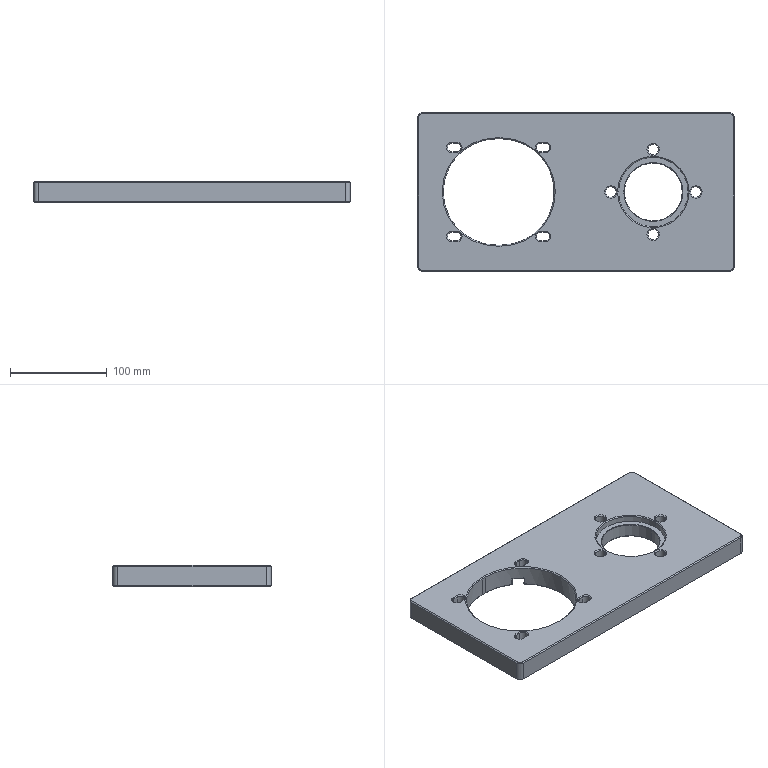NC program | NX | posted with a generic post | part box 328 x 164 x 22 mm
Lines 2955 to 3858 of 5416:
(ZLEVEL_PROFILE_1_COPY , TOOL : D3R0.5)
N5878 T05 M6
N5880 G54
N5882 G17 G0 G90 X124.56 Y41.708 S7000 M3
N5884 G43 Z30. H5
N5886 Z-7.
N5888 G94 G1 X128.387 Y41.707 Z-7.201 F2500.
N5890 X128.629 Y41.719 Z-7.213
N5892 X128.921 Y41.73 Z-7.229
N5894 X129.647 Y41.874 Z-7.267
N5896 X130.338 Y42.141 Z-7.306
N5898 X130.972 Y42.524 Z-7.345
N5900 X131.53 Y43.012 Z-7.384
N5902 X131.995 Y43.588 Z-7.423
N5904 X132.353 Y44.237 Z-7.461
N5906 X132.593 Y44.938 Z-7.5
N5908 X132.708 Y45.669 Z-7.539
N5910 Y46.253 Z-7.57
N5912 X132.593 Y46.984 Z-7.609
N5914 X132.353 Y47.685 Z-7.647
N5916 X131.995 Y48.334 Z-7.686
N5918 X131.53 Y48.91 Z-7.725
N5920 X130.972 Y49.398 Z-7.764
N5922 X130.338 Y49.781 Z-7.803
N5924 X129.647 Y50.048 Z-7.841
N5926 X128.921 Y50.192 Z-7.88
N5928 X128.629 Y50.203 Z-7.896
N5930 X128.387 Y50.216 Z-7.908
N5932 X125.962 Y50.217 Z-8.035
N5934 X123.537
N5936 X123.294 Y50.205
N5938 G3 X123.294 Y41.721 R4.245
N5940 G1 X123.537 Y41.708
N5942 X128.387 Y41.707
N5944 X128.629 Y41.719
N5946 G3 X128.629 Y50.203 R4.246
N5948 G1 X128.387 Y50.216
N5950 X125.962 Y50.217
N5952 X125.849 Y50.218 Z-8.037
N5954 X124.049 Y50.186 Z-8.069
N5956 X123.936 Y50.182 Z-8.071
N5958 X123.537
N5960 X123.294 Y50.17
N5962 G3 X123.294 Y41.755 R4.211
N5964 G1 X123.537 Y41.742
N5966 X128.387 Y41.741
N5968 X128.629 Y41.753
N5970 G3 X128.629 Y50.17 R4.212
N5972 G1 X128.387 Y50.182
N5974 X125.962
N5976 X125.849 Z-8.073
N5978 X124.049 Y50.151 Z-8.104
N5980 X123.936 Y50.148 Z-8.106
N5982 X123.537
N5984 X123.294 Y50.136
N5986 G3 X123.294 Y41.789 R4.177
N5988 G1 X123.537 Y41.776
N5990 X128.387
N5992 G3 X128.387 Y50.148 R-4.186
N5994 G1 X125.962
N5996 X125.849 Y50.147 Z-8.108
N5998 X124.049 Y50.115 Z-8.139
N6000 X123.936 Y50.113 Z-8.141
N6002 X123.537
N6004 G3 X123.537 Y41.811 R-4.152
N6006 G1 X128.387
N6008 G3 X128.387 Y50.113 R-4.152
N6010 G1 X125.962
N6012 X125.849 Y50.111 Z-8.143
N6014 X123.936 Y50.078 Z-8.177
N6016 X123.447
N6018 X123.052 Y50.058
N6020 G3 X123.462 Y41.846 R4.116
N6022 G1 X128.462
N6024 G3 X132.578 Y45.962 R4.116
N6026 X128.462 Y50.078 R4.116
N6028 G1 X125.962
N6030 X123.936 Y50.043 Z-8.212
N6032 X123.462
N6034 G3 X119.381 Y45.962 R4.081
N6036 X123.462 Y41.881 R4.081
N6038 G1 X128.462
N6040 G3 X132.543 Y45.962 R4.081
N6042 X128.462 Y50.043 R4.081
N6044 G1 X125.962
N6046 X123.936 Y50.007 Z-8.247
N6048 X123.462
N6050 G3 X119.417 Y45.962 R4.045
N6052 X123.462 Y41.917 R4.045
N6054 G1 X128.462
N6056 G3 X132.507 Y45.962 R4.045
N6058 X128.462 Y50.007 R4.045
N6060 G1 X125.962
N6062 X123.936 Y49.972 Z-8.283
N6064 X123.462
N6066 G3 X119.452 Y45.962 R4.01
N6068 X123.462 Y41.952 R4.01
N6070 G1 X128.462
N6072 G3 X132.472 Y45.962 R4.01
N6074 X128.462 Y49.972 R4.01
N6076 G1 X125.962
N6078 X123.936 Y49.937 Z-8.318
N6080 X123.462
N6082 G3 X119.487 Y45.962 R3.975
N6084 X123.462 Y41.987 R3.975
N6086 G1 X128.462
N6088 G3 X132.437 Y45.962 R3.975
N6090 X128.462 Y49.937 R3.975
N6092 G1 X125.962
N6094 X123.936 Y49.901 Z-8.354
N6096 X123.462
N6098 G3 X119.523 Y45.962 R3.939
N6100 X123.462 Y42.023 R3.939
N6102 G1 X128.462
N6104 G3 X132.401 Y45.962 R3.939
N6106 X128.462 Y49.901 R3.939
N6108 G1 X125.962
N6110 X123.936 Y49.866 Z-8.389
N6112 X123.462
N6114 G3 X119.558 Y45.962 R3.904
N6116 X123.462 Y42.058 R3.904
N6118 G1 X128.462
N6120 G3 X132.366 Y45.962 R3.904
N6122 X128.462 Y49.866 R3.904
N6124 G1 X125.962
N6126 X123.936 Y49.831 Z-8.424
N6128 X123.462
N6130 G3 X119.593 Y45.962 R3.869
N6132 X123.462 Y42.093 R3.869
N6134 G1 X128.462
N6136 G3 X132.331 Y45.962 R3.869
N6138 X128.462 Y49.831 R3.869
N6140 G1 X125.962
N6142 X123.936 Y49.795 Z-8.46
N6144 X123.462
N6146 G3 X119.629 Y45.962 R3.833
N6148 X123.462 Y42.129 R3.833
N6150 G1 X128.462
N6152 G3 X132.295 Y45.962 R3.833
N6154 X128.462 Y49.795 R3.833
N6156 G1 X125.962
N6158 X123.936 Y49.76 Z-8.495
N6160 X123.462
N6162 G3 X119.664 Y45.962 R3.798
N6164 X123.462 Y42.164 R3.798
N6166 G1 X128.462
N6168 G3 X132.26 Y45.962 R3.798
N6170 X128.462 Y49.76 R3.798
N6172 G1 X125.962
N6174 X123.936 Y49.725 Z-8.53
N6176 X123.462
N6178 G3 X119.699 Y45.962 R3.763
N6180 X123.462 Y42.199 R3.763
N6182 G1 X128.462
N6184 G3 X132.225 Y45.962 R3.763
N6186 X128.462 Y49.725 R3.763
N6188 G1 X125.962
N6190 X123.936 Y49.689 Z-8.566
N6192 X123.462
N6194 G3 X119.735 Y45.962 R3.727
N6196 X123.462 Y42.235 R3.727
N6198 G1 X128.462
N6200 G3 X132.189 Y45.962 R3.727
N6202 X128.462 Y49.689 R3.727
N6204 G1 X125.962
N6206 X123.936 Y49.654 Z-8.601
N6208 X123.462
N6210 G3 X119.77 Y45.962 R3.692
N6212 X123.462 Y42.27 R3.692
N6214 G1 X128.462
N6216 G3 X132.154 Y45.962 R3.692
N6218 X128.462 Y49.654 R3.692
N6220 G1 X125.962
N6222 X123.936 Y49.618 Z-8.636
N6224 X123.462
N6226 G3 X119.805 Y45.962 R3.656
N6228 X123.462 Y42.305 R3.656
N6230 G1 X128.462
N6232 G3 X132.118 Y45.962 R3.656
N6234 X128.462 Y49.618 R3.656
N6236 G1 X125.962
N6238 X123.936 Y49.583 Z-8.672
N6240 X123.462
N6242 G3 X119.841 Y45.962 R3.621
N6244 X123.462 Y42.341 R3.621
N6246 G1 X128.462
N6248 G3 X132.083 Y45.962 R3.621
N6250 X128.462 Y49.583 R3.621
N6252 G1 X125.962
N6254 X123.936 Y49.548 Z-8.707
N6256 X123.462
N6258 G3 X119.876 Y45.962 R3.586
N6260 X123.462 Y42.376 R3.586
N6262 G1 X128.462
N6264 G3 X132.048 Y45.962 R3.586
N6266 X128.462 Y49.548 R3.586
N6268 G1 X125.962
N6270 X123.936 Y49.512 Z-8.742
N6272 X123.462
N6274 G3 X119.912 Y45.962 R3.55
N6276 X123.462 Y42.412 R3.55
N6278 G1 X128.462
N6280 G3 X132.012 Y45.962 R3.55
N6282 X128.462 Y49.512 R3.55
N6284 G1 X125.962
N6286 X123.936 Y49.477 Z-8.778
N6288 X123.462
N6290 G3 X119.947 Y45.962 R3.515
N6292 X123.462 Y42.447 R3.515
N6294 G1 X128.462
N6296 G3 X131.977 Y45.962 R3.515
N6298 X128.462 Y49.477 R3.515
N6300 G1 X125.962
N6302 X123.936 Y49.442 Z-8.813
N6304 X123.462
N6306 G3 X119.982 Y45.962 R3.48
N6308 X123.462 Y42.482 R3.48
N6310 G1 X128.462
N6312 G3 X131.942 Y45.962 R3.48
N6314 X128.462 Y49.442 R3.48
N6316 G1 X125.962
N6318 X123.936 Y49.406 Z-8.849
N6320 X123.462
N6322 G3 X120.018 Y45.962 R3.444
N6324 X123.462 Y42.518 R3.444
N6326 G1 X128.462
N6328 G3 X131.906 Y45.962 R3.444
N6330 X128.462 Y49.406 R3.444
N6332 G1 X125.962
N6334 X123.936 Y49.371 Z-8.884
N6336 X123.462
N6338 G3 X120.053 Y45.962 R3.409
N6340 X123.462 Y42.553 R3.409
N6342 G1 X128.462
N6344 G3 X131.871 Y45.962 R3.409
N6346 X128.462 Y49.371 R3.409
N6348 G1 X125.962
N6350 X123.936 Y49.336 Z-8.919
N6352 X123.462
N6354 G3 X120.088 Y45.962 R3.374
N6356 X123.462 Y42.588 R3.374
N6358 G1 X128.462
N6360 G3 X131.836 Y45.962 R3.374
N6362 X128.462 Y49.336 R3.374
N6364 G1 X125.962
N6366 X123.936 Y49.3 Z-8.955
N6368 X123.462
N6370 G3 X120.124 Y45.962 R3.338
N6372 X123.462 Y42.624 R3.338
N6374 G1 X128.462
N6376 G3 X131.8 Y45.962 R3.338
N6378 X128.462 Y49.3 R3.338
N6380 G1 X125.962
N6382 X123.936 Y49.265 Z-8.99
N6384 X123.462
N6386 G3 X120.159 Y45.962 R3.303
N6388 X123.462 Y42.659 R3.303
N6390 G1 X128.462
N6392 G3 X131.765 Y45.962 R3.303
N6394 X128.462 Y49.265 R3.303
N6396 G1 X125.962
N6398 X123.936 Y49.23 Z-9.025
N6400 X123.462
N6402 G3 X120.194 Y45.962 R3.268
N6404 X123.462 Y42.694 R3.268
N6406 G1 X128.462
N6408 G3 X131.73 Y45.962 R3.268
N6410 X128.462 Y49.23 R3.268
N6412 G1 X125.962
N6414 X123.936 Y49.194 Z-9.061
N6416 X123.462
N6418 G3 X120.23 Y45.962 R3.232
N6420 X123.462 Y42.73 R3.232
N6422 G1 X128.462
N6424 G3 X131.694 Y45.962 R3.232
N6426 X128.462 Y49.194 R3.232
N6428 G1 X125.962
N6430 X123.936 Y49.159 Z-9.096
N6432 X123.462
N6434 G3 X120.265 Y45.962 R3.197
N6436 X123.462 Y42.765 R3.197
N6438 G1 X128.462
N6440 G3 X131.659 Y45.962 R3.197
N6442 X128.462 Y49.159 R3.197
N6444 G1 X125.962
N6446 X123.936 Y49.123 Z-9.131
N6448 X123.462
N6450 X123.386
N6452 X123.188 Y49.105
N6454 X123.145 Y49.108
N6456 G3 X120.882 Y47.79 R3.162
N6458 G1 X120.87 Y47.761
N6460 X120.726 Y47.547
N6462 X120.696 Y47.494
N6464 X120.552 Y47.198
N6466 G3 X120.592 Y44.637 R3.162
N6468 G1 X120.605 Y44.621
N6470 X120.683 Y44.466
N6472 X120.696 Y44.431
N6474 X120.763 Y44.315
N6476 X120.87 Y44.163
N6478 X120.882 Y44.134
N6480 G3 X123.462 Y42.8 R3.162
N6482 G1 X128.462
N6484 X128.549 Y42.802
N6486 X128.767 Y42.815
N6488 G3 X130.453 Y43.507 R3.162
N6490 G1 X130.686 Y43.715
N6492 X130.761 Y43.791
N6494 X130.946 Y44.006
N6496 G3 X131.613 Y45.701 R3.162
N6498 G1 X131.615 Y45.84
N6500 X131.622 Y45.854
N6502 X131.623 Y45.962
N6504 X131.603 Y46.32
N6506 G3 X130.875 Y48.005 R3.162
N6508 G1 X130.757 Y48.137
N6510 X130.628 Y48.265
N6512 X130.606 Y48.277
N6514 X130.359 Y48.491
N6516 G3 X128.763 Y49.109 R3.162
N6518 G1 X128.712 Y49.108
N6520 X128.462 Y49.123
N6522 X125.962
N6524 X125.174 Y49.11 Z-9.145
N6526 X125.062 Y49.108 Z-9.147
N6528 X124.949 Y49.106 Z-9.149
N6530 X124.837 Y49.104 Z-9.151
N6532 X124.724 Y49.101 Z-9.153
N6534 X124.612 Y49.1 Z-9.155
N6536 X124.499 Y49.097 Z-9.157
N6538 X124.387 Y49.095 Z-9.159
N6540 X124.274 Y49.093 Z-9.161
N6542 X124.162 Y49.091 Z-9.163
N6544 X124.049 Y49.089 Z-9.165
N6546 X123.936 Y49.087 Z-9.167
N6548 X123.456
N6550 G3 X123.273 Y42.852 R3.12
N6552 G1 X123.537 Y42.837
N6554 X128.387
N6556 G3 X128.387 Y49.087 R-3.126
N6558 G1 X125.962
N6560 X125.849 Y49.086 Z-9.169
N6562 X125.737 Y49.084 Z-9.171
N6564 X125.624 Y49.082 Z-9.173
N6566 X125.512 Y49.08 Z-9.175
N6568 X125.399 Y49.078 Z-9.177
N6570 X125.287 Y49.076 Z-9.179
N6572 X125.174 Y49.074 Z-9.18
N6574 X125.062 Y49.072 Z-9.182
N6576 X124.949 Y49.07 Z-9.184
N6578 X124.837 Y49.068 Z-9.186
N6580 X124.724 Y49.065 Z-9.188
N6582 X124.612 Y49.063 Z-9.19
N6584 X124.499 Y49.061 Z-9.192
N6586 X124.387 Y49.059 Z-9.194
N6588 X124.274 Y49.056 Z-9.196
N6590 X124.162 Y49.055 Z-9.198
N6592 X124.049 Y49.051 Z-9.2
N6594 X123.936 Y49.05 Z-9.202
N6596 X123.537 Y49.049
N6598 G3 X123.053 Y42.902 R3.088
N6600 X123.51 Y42.871 R3.403
N6602 G1 X128.458 Y42.874
N6604 G3 X131.545 Y45.964 R3.088
N6606 X128.469 Y49.05 R3.088
N6608 G1 X127.902 Y49.052
N6610 X125.962 Y49.051
N6612 X125.849 Y49.05 Z-9.204
N6614 X125.737 Y49.048 Z-9.206
N6616 X125.624 Y49.046 Z-9.208
N6618 X125.512 Y49.044 Z-9.21
N6620 X125.399 Y49.042 Z-9.212
N6622 X125.287 Y49.04 Z-9.214
N6624 X125.174 Y49.038 Z-9.216
N6626 X125.062 Y49.036 Z-9.218
N6628 X124.949 Y49.034 Z-9.22
N6630 X124.837 Y49.032 Z-9.222
N6632 X124.724 Y49.029 Z-9.224
N6634 X124.612 Y49.027 Z-9.226
N6636 X124.499 Y49.024 Z-9.228
N6638 X124.387 Y49.023 Z-9.23
N6640 X124.274 Y49.02 Z-9.232
N6642 X124.162 Y49.018 Z-9.234
N6644 X124.049 Y49.015 Z-9.235
N6646 X123.937 Y49.012 Z-9.237
N6648 X123.537
N6650 G3 X123.537 Y42.911 R-3.051
N6652 G1 X128.465
N6654 G3 X128.638 Y49.002 R3.048
N6656 X128.1 Y49.017 R9.302
N6658 G1 X125.962 Y49.015
N6660 X125.849 Z-9.239
N6662 X125.737 Y49.013 Z-9.241
N6664 X125.624 Y49.011 Z-9.243
N6666 X125.512 Y49.009 Z-9.245
N6668 X125.399 Y49.007 Z-9.247
N6670 X125.287 Y49.005 Z-9.249
N6672 X125.174 Y49.003 Z-9.251
N6674 X125.062 Y49.001 Z-9.253
N6676 X124.949 Y48.998 Z-9.255
N6678 X124.837 Y48.996 Z-9.257
N6680 X124.724 Y48.993 Z-9.259
N6682 X124.612 Y48.991 Z-9.261
N6684 X124.499 Y48.988 Z-9.263
N6686 X124.387 Y48.987 Z-9.265
N6688 X124.274 Y48.983 Z-9.267
N6690 X124.162 Y48.982 Z-9.269
N6692 X124.049 Y48.978 Z-9.271
N6694 X123.937 Y48.976 Z-9.273
N6696 X123.537 Y48.975
N6698 G3 X123.537 Y42.948 R-3.015
N6700 G1 X128.458
N6702 G3 X131.472 Y45.962 R3.014
N6704 X128.479 Y48.976 R3.014
N6706 G1 X127.902 Y48.98
N6708 X125.962 Y48.978
N6710 X125.85 Y48.979 Z-9.275
N6712 X125.737 Y48.977 Z-9.277
N6714 X125.624 Y48.975 Z-9.279
N6716 X125.512 Y48.973 Z-9.281
N6718 X125.399 Y48.971 Z-9.283
N6720 X125.287 Y48.969 Z-9.285
N6722 X125.174 Y48.967 Z-9.287
N6724 X125.062 Y48.965 Z-9.289
N6726 X124.949 Y48.962 Z-9.29
N6728 X124.837 Y48.96 Z-9.292
N6730 X124.724 Y48.957 Z-9.294
N6732 X124.612 Y48.955 Z-9.296
N6734 X124.499 Y48.952 Z-9.298
N6736 X124.387 Y48.95 Z-9.3
N6738 X124.274 Y48.947 Z-9.302
N6740 X124.162 Y48.946 Z-9.304
N6742 X124.049 Y48.942 Z-9.306
N6744 X123.937 Y48.938 Z-9.308
N6746 X123.464
N6748 G3 X120.489 Y45.961 R2.976
N6750 X123.442 Y42.985 R2.976
N6752 G1 X124.022 Y42.981
N6754 X128.387 Y42.984
N6756 G3 X128.387 Y48.94 R-2.979
N6758 G1 X125.962 Y48.939
N6760 X125.85 Y48.943 Z-9.31
N6762 X125.737 Y48.942 Z-9.312
N6764 X125.624 Y48.939 Z-9.314
N6766 X125.512 Y48.938 Z-9.316
N6768 X125.399 Y48.935 Z-9.318
N6770 X125.287 Y48.934 Z-9.32
N6772 X125.174 Y48.931 Z-9.322
N6774 X125.062 Y48.929 Z-9.324
N6776 X124.949 Y48.926 Z-9.326
N6778 X124.837 Y48.924 Z-9.328
N6780 X124.724 Y48.92 Z-9.33
N6782 X124.612 Y48.919 Z-9.332
N6784 X124.499 Y48.915 Z-9.334
N6786 X124.387 Y48.914 Z-9.336
N6788 X124.274 Y48.91 Z-9.338
N6790 X124.162 Z-9.34
N6792 X124.049 Y48.905 Z-9.342
N6794 X123.937 Y48.901 Z-9.344
N6796 X123.537
N6798 G3 X121.112 Y44.201 R2.938
N6800 X123.45 Y43.021 R2.907
N6802 G1 X128.387
N6804 G3 X128.387 Y48.903 R-2.942
N6806 G1 X125.962 Y48.902
N6808 X125.85 Y48.908 Z-9.345
N6810 X125.737 Y48.906 Z-9.347
N6812 X125.625 Y48.904 Z-9.349
N6814 X125.512 Y48.902 Z-9.351
N6816 X125.399 Y48.9 Z-9.353
N6818 X125.287 Y48.898 Z-9.355
N6820 X125.174 Y48.896 Z-9.357
N6822 X125.062 Y48.894 Z-9.359
N6824 X124.949 Y48.89 Z-9.361
N6826 X124.837 Y48.889 Z-9.363
N6828 X124.724 Y48.884 Z-9.365
N6830 X124.612 Z-9.367
N6832 X124.499 Y48.879 Z-9.369
N6834 X124.387 Y48.878 Z-9.371
N6836 X124.274 Y48.874 Z-9.373
N6838 X124.162 Y48.873 Z-9.375
N6840 X124.049 Y48.869 Z-9.377
N6842 X123.937 Y48.864 Z-9.379
N6844 X123.537
N6846 G3 X123.537 Y43.058 R-2.904
N6848 G1 X128.387 Y43.057
N6850 G3 X128.387 Y48.866 R-2.905
N6852 G1 X125.962 Y48.865
N6854 X125.85 Y48.872 Z-9.381
N6856 X125.737 Y48.871 Z-9.383
N6858 X125.625 Y48.868 Z-9.385
N6860 X125.512 Y48.867 Z-9.387
N6862 X125.399 Y48.864 Z-9.389
N6864 X125.287 Y48.863 Z-9.391
N6866 X125.174 Y48.86 Z-9.393
N6868 X125.062 Y48.858 Z-9.395
N6870 X124.949 Y48.854 Z-9.397
N6872 X124.837 Y48.853 Z-9.399
N6874 X124.724 Y48.848 Z-9.4
N6876 X124.612 Z-9.402
N6878 X124.499 Y48.843 Z-9.404
N6880 X124.387 Y48.842 Z-9.406
N6882 X124.274 Y48.837 Z-9.408
N6884 X124.162 Z-9.41
N6886 X124.049 Y48.832 Z-9.412
N6888 X123.937 Y48.828 Z-9.414
N6890 X123.461 Y48.827
N6892 G3 X120.599 Y45.957 R2.866
N6894 X123.464 Y43.095 R2.866
N6896 G1 X128.458 Y43.094
N6898 G3 X131.326 Y45.961 R2.868
N6900 X128.48 Y48.829 R2.868
N6902 G1 X127.902 Y48.833
N6904 X125.962 Y48.831
N6906 X125.85 Y48.837 Z-9.416
N6908 X125.737 Y48.835 Z-9.418
N6910 X125.625 Y48.833 Z-9.42
N6912 X125.512 Y48.831 Z-9.422
N6914 X125.4 Y48.829 Z-9.424
N6916 X125.287 Y48.827 Z-9.426
N6918 X125.174 Y48.825 Z-9.428
N6920 X125.062 Y48.822 Z-9.43
N6922 X124.949 Y48.819 Z-9.432
N6924 X124.837 Y48.817 Z-9.434
N6926 X124.724 Y48.813 Z-9.436
N6928 X124.612 Y48.811 Z-9.438
N6930 X124.499 Y48.807 Z-9.44
N6932 X124.387 Y48.806 Z-9.442
N6934 X124.274 Y48.801 Z-9.444
N6936 X124.162 Z-9.446
N6938 X124.049 Y48.795 Z-9.448
N6940 X123.937 Y48.791 Z-9.45
N6942 X123.46 Y48.79
N6944 G3 X123.438 Y43.133 R2.829
N6946 G1 X123.779 Y43.13
N6948 X128.46 Y43.131
N6950 G3 X131.29 Y45.962 R2.831
N6952 X128.481 Y48.792 R2.831
N6954 G1 X127.902 Y48.797
N6956 X125.962 Y48.794
N6958 X125.85 Y48.801 Z-9.452
N6960 X125.737 Y48.8 Z-9.453
N6962 X125.625 Y48.797 Z-9.455
N6964 X125.512 Y48.796 Z-9.457
N6966 X125.4 Y48.793 Z-9.459
N6968 X125.287 Y48.791 Z-9.461
N6970 X125.175 Y48.789 Z-9.463
N6972 X125.062 Y48.787 Z-9.465
N6974 X124.949 Y48.783 Z-9.467
N6976 X124.837 Y48.781 Z-9.469
N6978 X124.724 Y48.777 Z-9.471
N6980 X124.612 Y48.775 Z-9.473
N6982 X124.499 Y48.771 Z-9.475
N6984 X124.387 Y48.77 Z-9.477
N6986 X124.274 Y48.765 Z-9.479
N6988 X124.162 Y48.764 Z-9.481
N6990 X124.049 Y48.76 Z-9.483
N6992 X123.937 Y48.758 Z-9.485
N6994 G3 X123.537 Y48.754 R215.595
N6996 G1 X123.052 Y48.727
N6998 G3 X120.803 Y45.109 R2.798
N7000 X123.052 Y43.198 R2.798
N7002 G1 X123.294 Y43.179
N7004 X123.537 Y43.169
N7006 G3 X128.494 Y43.168 R230.884
N7008 X131.054 Y44.915 R2.793
N7010 X128.489 Y48.755 R2.798
N7012 X125.962 Y48.769 R215.595
N7014 G1 X125.854 Y48.766 Z-9.487
N7016 X125.746 Y48.764 Z-9.489
N7018 X125.638 Y48.762 Z-9.491
N7020 X125.53 Y48.76 Z-9.492
N7022 X125.422 Y48.758 Z-9.494
N7024 X125.314 Y48.756 Z-9.496
N7026 X125.207 Y48.754 Z-9.498
N7028 X125.099 Y48.75 Z-9.5
N7030 G3 X123.294 Y48.728 R165.123
N7032 X121.112 Y47.42 R2.659
N7034 X121.042 Y44.621 R2.662
N7036 X123.369 Y43.193 R2.688
N7038 X128.629 Y43.191 R148.755
N7040 X130.569 Y47.764 R2.772
N7042 X128.519 Y48.74 R2.72
N7044 X125.099 Y48.75 R165.123
N7046 G1 Z-8.5
N7048 G0 Z30.
N7050 X32.636 Y41.708
N7052 Z-7.
N7054 G1 X36.463 Y41.707 Z-7.201
N7056 X36.706 Y41.719 Z-7.213
N7058 X36.997 Y41.73 Z-7.229
N7060 X37.724 Y41.874 Z-7.267
N7062 X38.414 Y42.141 Z-7.306
N7064 X39.048 Y42.524 Z-7.345
N7066 X39.606 Y43.012 Z-7.384
N7068 X40.071 Y43.588 Z-7.423
N7070 X40.429 Y44.237 Z-7.461
N7072 X40.669 Y44.938 Z-7.5
N7074 X40.784 Y45.669 Z-7.539
N7076 Y46.253 Z-7.57
N7078 X40.669 Y46.984 Z-7.609
N7080 X40.429 Y47.685 Z-7.647
N7082 X40.071 Y48.334 Z-7.686
N7084 X39.606 Y48.91 Z-7.725
N7086 X39.048 Y49.398 Z-7.764
N7088 X38.414 Y49.781 Z-7.803
N7090 X37.724 Y50.048 Z-7.841
N7092 X36.997 Y50.192 Z-7.88
N7094 X36.706 Y50.203 Z-7.896
N7096 X36.463 Y50.216 Z-7.908
N7098 X34.038 Y50.217 Z-8.035
N7100 X31.613
N7102 X31.371 Y50.205
N7104 G3 X31.371 Y41.721 R4.245
N7106 G1 X31.613 Y41.708
N7108 X36.463 Y41.707
N7110 X36.706 Y41.719
N7112 G3 X36.706 Y50.203 R4.246
N7114 G1 X36.463 Y50.216
N7116 X34.038 Y50.217
N7118 X33.926 Y50.218 Z-8.037
N7120 X32.125 Y50.186 Z-8.069
N7122 X32.013 Y50.182 Z-8.071
N7124 X31.613
N7126 X31.371 Y50.17
N7128 G3 X31.371 Y41.755 R4.211
N7130 G1 X31.613 Y41.742
N7132 X36.463 Y41.741
N7134 X36.706 Y41.753
N7136 G3 X36.706 Y50.17 R4.212
N7138 G1 X36.463 Y50.182
N7140 X34.038
N7142 X33.926 Z-8.073
N7144 X32.125 Y50.151 Z-8.104
N7146 X32.013 Y50.148 Z-8.106
N7148 X31.613
N7150 X31.371 Y50.136
N7152 G3 X31.371 Y41.789 R4.177
N7154 G1 X31.613 Y41.776
N7156 X36.463
N7158 G3 X36.463 Y50.148 R-4.186
N7160 G1 X34.038
N7162 X33.926 Y50.147 Z-8.108
N7164 X32.125 Y50.115 Z-8.139
N7166 X32.013 Y50.113 Z-8.141
N7168 X31.613
N7170 G3 X31.613 Y41.811 R-4.152
N7172 G1 X36.463
N7174 G3 X36.463 Y50.113 R-4.152
N7176 G1 X34.038
N7178 X33.926 Y50.111 Z-8.143
N7180 X32.013 Y50.078 Z-8.177
N7182 X31.523
N7184 X31.128 Y50.058
N7186 G3 X31.538 Y41.846 R4.116
N7188 G1 X36.538
N7190 G3 X40.654 Y45.962 R4.116
N7192 X36.538 Y50.078 R4.116
N7194 G1 X34.038
N7196 X32.013 Y50.043 Z-8.212
N7198 X31.538
N7200 G3 X27.457 Y45.962 R4.081
N7202 X31.538 Y41.881 R4.081
N7204 G1 X36.538
N7206 G3 X40.619 Y45.962 R4.081
N7208 X36.538 Y50.043 R4.081
N7210 G1 X34.038
N7212 X32.013 Y50.007 Z-8.247
N7214 X31.538
N7216 G3 X27.493 Y45.962 R4.045
N7218 X31.538 Y41.917 R4.045
N7220 G1 X36.538
N7222 G3 X40.583 Y45.962 R4.045
N7224 X36.538 Y50.007 R4.045
N7226 G1 X34.038
N7228 X32.013 Y49.972 Z-8.283
N7230 X31.538
N7232 G3 X27.528 Y45.962 R4.01
N7234 X31.538 Y41.952 R4.01
N7236 G1 X36.538
N7238 G3 X40.548 Y45.962 R4.01
N7240 X36.538 Y49.972 R4.01
N7242 G1 X34.038
N7244 X32.013 Y49.937 Z-8.318
N7246 X31.538
N7248 G3 X27.563 Y45.962 R3.975
N7250 X31.538 Y41.987 R3.975
N7252 G1 X36.538
N7254 G3 X40.513 Y45.962 R3.975
N7256 X36.538 Y49.937 R3.975
N7258 G1 X34.038
N7260 X32.013 Y49.901 Z-8.354
N7262 X31.538
N7264 G3 X27.599 Y45.962 R3.939
N7266 X31.538 Y42.023 R3.939
N7268 G1 X36.538
N7270 G3 X40.477 Y45.962 R3.939
N7272 X36.538 Y49.901 R3.939
N7274 G1 X34.038
N7276 X32.013 Y49.866 Z-8.389
N7278 X31.538
N7280 G3 X27.634 Y45.962 R3.904
N7282 X31.538 Y42.058 R3.904
N7284 G1 X36.538
N7286 G3 X40.442 Y45.962 R3.904
N7288 X36.538 Y49.866 R3.904
N7290 G1 X34.038
N7292 X32.013 Y49.831 Z-8.424
N7294 X31.538
N7296 G3 X27.669 Y45.962 R3.869
N7298 X31.538 Y42.093 R3.869
N7300 G1 X36.538
N7302 G3 X40.407 Y45.962 R3.869
N7304 X36.538 Y49.831 R3.869
N7306 G1 X34.038
N7308 X32.013 Y49.795 Z-8.46
N7310 X31.538
N7312 G3 X27.705 Y45.962 R3.833
N7314 X31.538 Y42.129 R3.833
N7316 G1 X36.538
N7318 G3 X40.371 Y45.962 R3.833
N7320 X36.538 Y49.795 R3.833
N7322 G1 X34.038
N7324 X32.013 Y49.76 Z-8.495
N7326 X31.538
N7328 G3 X27.74 Y45.962 R3.798
N7330 X31.538 Y42.164 R3.798
N7332 G1 X36.538
N7334 G3 X40.336 Y45.962 R3.798
N7336 X36.538 Y49.76 R3.798
N7338 G1 X34.038
N7340 X32.013 Y49.725 Z-8.53
N7342 X31.538
N7344 G3 X27.775 Y45.962 R3.763
N7346 X31.538 Y42.199 R3.763
N7348 G1 X36.538
N7350 G3 X40.301 Y45.962 R3.763
N7352 X36.538 Y49.725 R3.763
N7354 G1 X34.038
N7356 X32.013 Y49.689 Z-8.566
N7358 X31.538
N7360 G3 X27.811 Y45.962 R3.727
N7362 X31.538 Y42.235 R3.727
N7364 G1 X36.538
N7366 G3 X40.265 Y45.962 R3.727
N7368 X36.538 Y49.689 R3.727
N7370 G1 X34.038
N7372 X32.013 Y49.654 Z-8.601
N7374 X31.538
N7376 G3 X27.846 Y45.962 R3.692
N7378 X31.538 Y42.27 R3.692
N7380 G1 X36.538
N7382 G3 X40.23 Y45.962 R3.692
N7384 X36.538 Y49.654 R3.692
N7386 G1 X34.038
N7388 X32.013 Y49.618 Z-8.636
N7390 X31.538
N7392 G3 X27.882 Y45.962 R3.656
N7394 X31.538 Y42.305 R3.656
N7396 G1 X36.538
N7398 G3 X40.195 Y45.962 R3.656
N7400 X36.538 Y49.618 R3.656
N7402 G1 X34.038
N7404 X32.013 Y49.583 Z-8.672
N7406 X31.538
N7408 G3 X27.917 Y45.962 R3.621
N7410 X31.538 Y42.341 R3.621
N7412 G1 X36.538
N7414 G3 X40.159 Y45.962 R3.621
N7416 X36.538 Y49.583 R3.621
N7418 G1 X34.038
N7420 X32.013 Y49.548 Z-8.707
N7422 X31.538
N7424 G3 X27.952 Y45.962 R3.586
N7426 X31.538 Y42.376 R3.586
N7428 G1 X36.538
N7430 G3 X40.124 Y45.962 R3.586
N7432 X36.538 Y49.548 R3.586
N7434 G1 X34.038
N7436 X32.013 Y49.512 Z-8.742
N7438 X31.538
N7440 G3 X27.988 Y45.962 R3.55
N7442 X31.538 Y42.412 R3.55
N7444 G1 X36.538
N7446 G3 X40.088 Y45.962 R3.55
N7448 X36.538 Y49.512 R3.55
N7450 G1 X34.038
N7452 X32.013 Y49.477 Z-8.778
N7454 X31.538
N7456 G3 X28.023 Y45.962 R3.515
N7458 X31.538 Y42.447 R3.515
N7460 G1 X36.538
N7462 G3 X40.053 Y45.962 R3.515
N7464 X36.538 Y49.477 R3.515
N7466 G1 X34.038
N7468 X32.013 Y49.442 Z-8.813
N7470 X31.538
N7472 G3 X28.058 Y45.962 R3.48
N7474 X31.538 Y42.482 R3.48
N7476 G1 X36.538
N7478 G3 X40.018 Y45.962 R3.48
N7480 X36.538 Y49.442 R3.48
N7482 G1 X34.038
N7484 X32.013 Y49.406 Z-8.849
N7486 X31.538
N7488 G3 X28.094 Y45.962 R3.444
N7490 X31.538 Y42.518 R3.444
N7492 G1 X36.538
N7494 G3 X39.982 Y45.962 R3.444
N7496 X36.538 Y49.406 R3.444
N7498 G1 X34.038
N7500 X32.013 Y49.371 Z-8.884
N7502 X31.538
N7504 G3 X28.129 Y45.962 R3.409
N7506 X31.538 Y42.553 R3.409
N7508 G1 X36.538
N7510 G3 X39.947 Y45.962 R3.409
N7512 X36.538 Y49.371 R3.409
N7514 G1 X34.038
N7516 X32.013 Y49.336 Z-8.919
N7518 X31.538
N7520 G3 X28.164 Y45.962 R3.374
N7522 X31.538 Y42.588 R3.374
N7524 G1 X36.538
N7526 G3 X39.912 Y45.962 R3.374
N7528 X36.538 Y49.336 R3.374
N7530 G1 X34.038
N7532 X32.013 Y49.3 Z-8.955
N7534 X31.538
N7536 G3 X28.2 Y45.962 R3.338
N7538 X31.538 Y42.624 R3.338
N7540 G1 X36.538
N7542 G3 X39.876 Y45.962 R3.338
N7544 X36.538 Y49.3 R3.338
N7546 G1 X34.038
N7548 X32.013 Y49.265 Z-8.99
N7550 X31.538
N7552 G3 X28.235 Y45.962 R3.303
N7554 X31.538 Y42.659 R3.303
N7556 G1 X36.538
N7558 G3 X39.841 Y45.962 R3.303
N7560 X36.538 Y49.265 R3.303
N7562 G1 X34.038
N7564 X32.013 Y49.23 Z-9.025
N7566 X31.538
N7568 G3 X28.27 Y45.962 R3.268
N7570 X31.538 Y42.694 R3.268
N7572 G1 X36.538
N7574 G3 X39.806 Y45.962 R3.268
N7576 X36.538 Y49.23 R3.268
N7578 G1 X34.038
N7580 X32.013 Y49.194 Z-9.061
N7582 X31.538
N7584 G3 X28.306 Y45.962 R3.232
N7586 X31.538 Y42.73 R3.232
N7588 G1 X36.538
N7590 G3 X39.77 Y45.962 R3.232
N7592 X36.538 Y49.194 R3.232
N7594 G1 X34.038
N7596 X32.013 Y49.159 Z-9.096
N7598 X31.538
N7600 G3 X28.341 Y45.962 R3.197
N7602 X31.538 Y42.765 R3.197
N7604 G1 X36.538
N7606 G3 X39.735 Y45.962 R3.197
N7608 X36.538 Y49.159 R3.197
N7610 G1 X34.038
N7612 X32.013 Y49.123 Z-9.131
N7614 X31.538
N7616 X31.461
N7618 X31.264 Y49.105
N7620 X31.221 Y49.108
N7622 G3 X28.959 Y47.79 R3.162
N7624 G1 X28.946 Y47.761
N7626 X28.802 Y47.547
N7628 X28.772 Y47.494
N7630 X28.633 Y47.209
N7632 G3 X28.668 Y44.637 R3.162
N7634 G1 X28.681 Y44.621
N7636 X28.759 Y44.466
N7638 X28.772 Y44.431
N7640 X28.839 Y44.315
N7642 X28.946 Y44.163
N7644 X28.959 Y44.134
N7646 G3 X31.538 Y42.8 R3.162
N7648 G1 X36.538
N7650 X36.625 Y42.802
N7652 X36.843 Y42.815
N7654 G3 X38.53 Y43.507 R3.162
N7656 G1 X38.762 Y43.715
N7658 X38.837 Y43.791
N7660 X39.022 Y44.006
N7662 G3 X39.689 Y45.701 R3.162
N7664 G1 X39.691 Y45.84
N7666 X39.698 Y45.854
N7668 X39.7 Y45.962
N7670 X39.679 Y46.32
N7672 G3 X38.951 Y48.005 R3.162
N7674 G1 X38.833 Y48.137
N7676 X38.704 Y48.265
N7678 X38.682 Y48.277